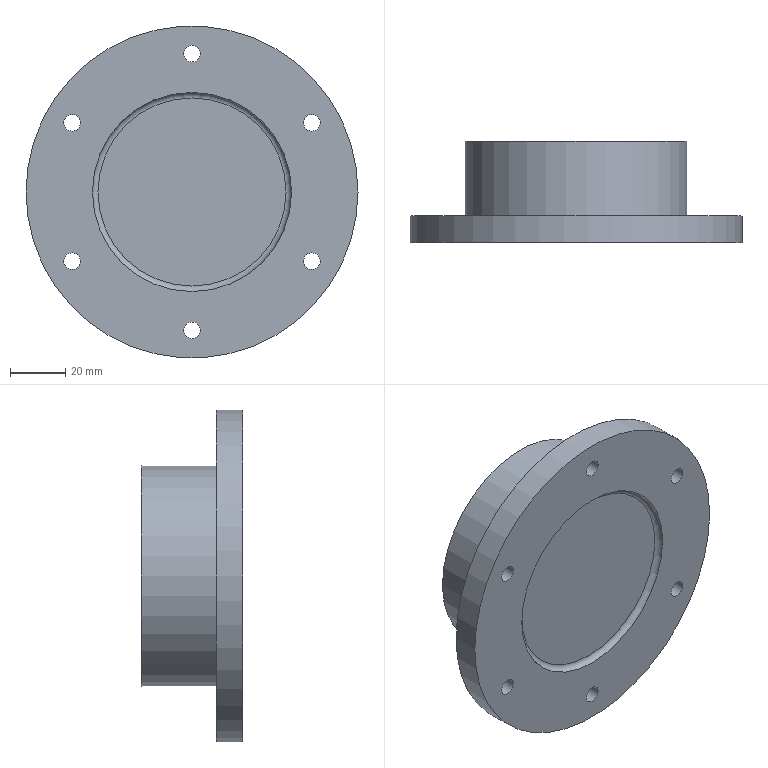Part | NX | features DATUM_CSYS 9, HOLE PACKAGE 9, SIMPLE HOLE 9, SKETCH 8, EXTRACT_DATUM_AXIS 6, EXTRACT_FACE 6, Instance Feature 5, BLEND 2, EXTRUDE 2, DELETE FACE 1, Pattern Feature 1 | 1 solid | 16 faces | box 120 x 36.6 x 120 mm | volume 144277 mm3 | cylinder 9 | plane 5 | torus 2 | commonest cylinder face diameters 6 x6 72 x1 80 x1 120 x1
STEP:
#1=CARTESIAN_POINT('',(60.,0.,0.));
#2=VERTEX_POINT('',#1);
#3=CARTESIAN_POINT('',(0.,0.,0.));
#4=DIRECTION('',(0.,-1.,0.));
#5=DIRECTION('',(1.,0.,0.));
#6=AXIS2_PLACEMENT_3D('',#3,#4,#5);
#7=CIRCLE('',#6,60.);
#8=EDGE_CURVE('',#2,#2,#7,.T.);
#9=ORIENTED_EDGE('',*,*,#8,.T.);
#10=EDGE_LOOP('',(#9));
#11=FACE_BOUND('',#10,.T.);
#12=CARTESIAN_POINT('',(60.,-9.6,0.));
#13=VERTEX_POINT('',#12);
#14=CARTESIAN_POINT('',(0.,-9.6,0.));
#15=DIRECTION('',(0.,-1.,0.));
#16=DIRECTION('',(1.,0.,0.));
#17=AXIS2_PLACEMENT_3D('',#14,#15,#16);
#18=CIRCLE('',#17,60.);
#19=EDGE_CURVE('',#13,#13,#18,.T.);
#20=ORIENTED_EDGE('',*,*,#19,.F.);
#21=EDGE_LOOP('',(#20));
#22=FACE_BOUND('',#21,.T.);
#23=CARTESIAN_POINT('',(0.,0.,0.));
#24=DIRECTION('',(0.,-1.,0.));
#25=DIRECTION('',(0.,0.,-1.));
#26=AXIS2_PLACEMENT_3D('',#23,#24,#25);
#27=CYLINDRICAL_SURFACE('',#26,60.);
#28=ADVANCED_FACE('',(#11,#22),#27,.T.);
#29=CARTESIAN_POINT('',(-43.301,0.,22.));
#30=VERTEX_POINT('',#29);
#31=CARTESIAN_POINT('',(-43.301,0.,25.));
#32=DIRECTION('',(0.,-1.,0.));
#33=DIRECTION('',(0.,0.,-1.));
#34=AXIS2_PLACEMENT_3D('',#31,#32,#33);
#35=CIRCLE('',#34,3.);
#36=EDGE_CURVE('',#30,#30,#35,.T.);
#37=ORIENTED_EDGE('',*,*,#36,.T.);
#38=EDGE_LOOP('',(#37));
#39=FACE_BOUND('',#38,.T.);
#40=CARTESIAN_POINT('',(-43.301,0.,-28.));
#41=VERTEX_POINT('',#40);
#42=CARTESIAN_POINT('',(-43.301,0.,-25.));
#43=DIRECTION('',(0.,-1.,0.));
#44=DIRECTION('',(0.,0.,-1.));
#45=AXIS2_PLACEMENT_3D('',#42,#43,#44);
#46=CIRCLE('',#45,3.);
#47=EDGE_CURVE('',#41,#41,#46,.T.);
#48=ORIENTED_EDGE('',*,*,#47,.T.);
#49=EDGE_LOOP('',(#48));
#50=FACE_BOUND('',#49,.T.);
#51=CARTESIAN_POINT('',(0.,0.,-53.));
#52=VERTEX_POINT('',#51);
#53=CARTESIAN_POINT('',(0.,0.,-50.));
#54=DIRECTION('',(0.,-1.,0.));
#55=DIRECTION('',(0.,0.,-1.));
#56=AXIS2_PLACEMENT_3D('',#53,#54,#55);
#57=CIRCLE('',#56,3.);
#58=EDGE_CURVE('',#52,#52,#57,.T.);
#59=ORIENTED_EDGE('',*,*,#58,.T.);
#60=EDGE_LOOP('',(#59));
#61=FACE_BOUND('',#60,.T.);
#62=CARTESIAN_POINT('',(43.301,0.,-28.));
#63=VERTEX_POINT('',#62);
#64=CARTESIAN_POINT('',(43.301,0.,-25.));
#65=DIRECTION('',(0.,-1.,0.));
#66=DIRECTION('',(0.,0.,-1.));
#67=AXIS2_PLACEMENT_3D('',#64,#65,#66);
#68=CIRCLE('',#67,3.);
#69=EDGE_CURVE('',#63,#63,#68,.T.);
#70=ORIENTED_EDGE('',*,*,#69,.T.);
#71=EDGE_LOOP('',(#70));
#72=FACE_BOUND('',#71,.T.);
#73=CARTESIAN_POINT('',(43.301,0.,22.));
#74=VERTEX_POINT('',#73);
#75=CARTESIAN_POINT('',(43.301,0.,25.));
#76=DIRECTION('',(0.,-1.,0.));
#77=DIRECTION('',(0.,0.,-1.));
#78=AXIS2_PLACEMENT_3D('',#75,#76,#77);
#79=CIRCLE('',#78,3.);
#80=EDGE_CURVE('',#74,#74,#79,.T.);
#81=ORIENTED_EDGE('',*,*,#80,.T.);
#82=EDGE_LOOP('',(#81));
#83=FACE_BOUND('',#82,.T.);
#84=CARTESIAN_POINT('',(0.,0.,47.));
#85=VERTEX_POINT('',#84);
#86=CARTESIAN_POINT('',(0.,0.,50.));
#87=DIRECTION('',(0.,-1.,0.));
#88=DIRECTION('',(0.,0.,-1.));
#89=AXIS2_PLACEMENT_3D('',#86,#87,#88);
#90=CIRCLE('',#89,3.);
#91=EDGE_CURVE('',#85,#85,#90,.T.);
#92=ORIENTED_EDGE('',*,*,#91,.T.);
#93=EDGE_LOOP('',(#92));
#94=FACE_BOUND('',#93,.T.);
#95=CARTESIAN_POINT('',(40.,0.,0.));
#96=VERTEX_POINT('',#95);
#97=CARTESIAN_POINT('',(0.,0.,0.));
#98=DIRECTION('',(0.,1.,0.));
#99=DIRECTION('',(1.,0.,0.));
#100=AXIS2_PLACEMENT_3D('',#97,#98,#99);
#101=CIRCLE('',#100,40.);
#102=EDGE_CURVE('',#96,#96,#101,.T.);
#103=ORIENTED_EDGE('',*,*,#102,.F.);
#104=EDGE_LOOP('',(#103));
#105=FACE_BOUND('',#104,.T.);
#106=ORIENTED_EDGE('',*,*,#8,.F.);
#107=EDGE_LOOP('',(#106));
#108=FACE_BOUND('',#107,.T.);
#109=CARTESIAN_POINT('',(0.,0.,0.));
#110=DIRECTION('',(0.,-1.,0.));
#111=DIRECTION('',(0.,0.,-1.));
#112=AXIS2_PLACEMENT_3D('',#109,#110,#111);
#113=PLANE('',#112);
#114=ADVANCED_FACE('',(#39,#50,#61,#72,#83,#94,#105,#108),#113,.F.);
#115=CARTESIAN_POINT('',(-43.301,-9.6,28.));
#116=VERTEX_POINT('',#115);
#117=CARTESIAN_POINT('',(-43.301,-9.6,25.));
#118=DIRECTION('',(0.,1.,0.));
#119=DIRECTION('',(0.,0.,1.));
#120=AXIS2_PLACEMENT_3D('',#117,#118,#119);
#121=CIRCLE('',#120,3.);
#122=EDGE_CURVE('',#116,#116,#121,.T.);
#123=ORIENTED_EDGE('',*,*,#122,.T.);
#124=EDGE_LOOP('',(#123));
#125=FACE_BOUND('',#124,.T.);
#126=CARTESIAN_POINT('',(-43.301,-9.6,-22.));
#127=VERTEX_POINT('',#126);
#128=CARTESIAN_POINT('',(-43.301,-9.6,-25.));
#129=DIRECTION('',(0.,1.,0.));
#130=DIRECTION('',(0.,0.,1.));
#131=AXIS2_PLACEMENT_3D('',#128,#129,#130);
#132=CIRCLE('',#131,3.);
#133=EDGE_CURVE('',#127,#127,#132,.T.);
#134=ORIENTED_EDGE('',*,*,#133,.T.);
#135=EDGE_LOOP('',(#134));
#136=FACE_BOUND('',#135,.T.);
#137=CARTESIAN_POINT('',(0.,-9.6,-47.));
#138=VERTEX_POINT('',#137);
#139=CARTESIAN_POINT('',(0.,-9.6,-50.));
#140=DIRECTION('',(0.,1.,0.));
#141=DIRECTION('',(0.,0.,1.));
#142=AXIS2_PLACEMENT_3D('',#139,#140,#141);
#143=CIRCLE('',#142,3.);
#144=EDGE_CURVE('',#138,#138,#143,.T.);
#145=ORIENTED_EDGE('',*,*,#144,.T.);
#146=EDGE_LOOP('',(#145));
#147=FACE_BOUND('',#146,.T.);
#148=CARTESIAN_POINT('',(43.301,-9.6,-22.));
#149=VERTEX_POINT('',#148);
#150=CARTESIAN_POINT('',(43.301,-9.6,-25.));
#151=DIRECTION('',(0.,1.,0.));
#152=DIRECTION('',(0.,0.,1.));
#153=AXIS2_PLACEMENT_3D('',#150,#151,#152);
#154=CIRCLE('',#153,3.);
#155=EDGE_CURVE('',#149,#149,#154,.T.);
#156=ORIENTED_EDGE('',*,*,#155,.T.);
#157=EDGE_LOOP('',(#156));
#158=FACE_BOUND('',#157,.T.);
#159=CARTESIAN_POINT('',(43.301,-9.6,28.));
#160=VERTEX_POINT('',#159);
#161=CARTESIAN_POINT('',(43.301,-9.6,25.));
#162=DIRECTION('',(0.,1.,0.));
#163=DIRECTION('',(0.,0.,1.));
#164=AXIS2_PLACEMENT_3D('',#161,#162,#163);
#165=CIRCLE('',#164,3.);
#166=EDGE_CURVE('',#160,#160,#165,.T.);
#167=ORIENTED_EDGE('',*,*,#166,.T.);
#168=EDGE_LOOP('',(#167));
#169=FACE_BOUND('',#168,.T.);
#170=CARTESIAN_POINT('',(0.,-9.6,53.));
#171=VERTEX_POINT('',#170);
#172=CARTESIAN_POINT('',(0.,-9.6,50.));
#173=DIRECTION('',(0.,1.,0.));
#174=DIRECTION('',(0.,0.,1.));
#175=AXIS2_PLACEMENT_3D('',#172,#173,#174);
#176=CIRCLE('',#175,3.);
#177=EDGE_CURVE('',#171,#171,#176,.T.);
#178=ORIENTED_EDGE('',*,*,#177,.T.);
#179=EDGE_LOOP('',(#178));
#180=FACE_BOUND('',#179,.T.);
#181=CARTESIAN_POINT('',(0.,-9.6,36.));
#182=VERTEX_POINT('',#181);
#183=CARTESIAN_POINT('',(0.,-9.6,0.));
#184=DIRECTION('',(0.,1.,0.));
#185=DIRECTION('',(0.,0.,1.));
#186=AXIS2_PLACEMENT_3D('',#183,#184,#185);
#187=CIRCLE('',#186,36.);
#188=EDGE_CURVE('',#182,#182,#187,.T.);
#189=ORIENTED_EDGE('',*,*,#188,.T.);
#190=EDGE_LOOP('',(#189));
#191=FACE_BOUND('',#190,.T.);
#192=ORIENTED_EDGE('',*,*,#19,.T.);
#193=EDGE_LOOP('',(#192));
#194=FACE_BOUND('',#193,.T.);
#195=CARTESIAN_POINT('',(0.,-9.6,0.));
#196=DIRECTION('',(0.,-1.,0.));
#197=DIRECTION('',(0.,0.,-1.));
#198=AXIS2_PLACEMENT_3D('',#195,#196,#197);
#199=PLANE('',#198);
#200=ADVANCED_FACE('',(#125,#136,#147,#158,#169,#180,#191,#194),#199,.T.);
#201=ORIENTED_EDGE('',*,*,#102,.T.);
#202=EDGE_LOOP('',(#201));
#203=FACE_BOUND('',#202,.T.);
#204=CARTESIAN_POINT('',(40.,27.,0.));
#205=VERTEX_POINT('',#204);
#206=CARTESIAN_POINT('',(0.,27.,0.));
#207=DIRECTION('',(0.,1.,0.));
#208=DIRECTION('',(1.,0.,0.));
#209=AXIS2_PLACEMENT_3D('',#206,#207,#208);
#210=CIRCLE('',#209,40.);
#211=EDGE_CURVE('',#205,#205,#210,.T.);
#212=ORIENTED_EDGE('',*,*,#211,.F.);
#213=EDGE_LOOP('',(#212));
#214=FACE_BOUND('',#213,.T.);
#215=CARTESIAN_POINT('',(0.,0.,0.));
#216=DIRECTION('',(0.,1.,0.));
#217=DIRECTION('',(0.,0.,1.));
#218=AXIS2_PLACEMENT_3D('',#215,#216,#217);
#219=CYLINDRICAL_SURFACE('',#218,40.);
#220=ADVANCED_FACE('',(#203,#214),#219,.T.);
#221=CARTESIAN_POINT('',(0.,27.,-36.));
#222=VERTEX_POINT('',#221);
#223=CARTESIAN_POINT('',(0.,27.,0.));
#224=DIRECTION('',(0.,-1.,0.));
#225=DIRECTION('',(0.,0.,-1.));
#226=AXIS2_PLACEMENT_3D('',#223,#224,#225);
#227=CIRCLE('',#226,36.);
#228=EDGE_CURVE('',#222,#222,#227,.T.);
#229=ORIENTED_EDGE('',*,*,#228,.T.);
#230=EDGE_LOOP('',(#229));
#231=FACE_BOUND('',#230,.T.);
#232=ORIENTED_EDGE('',*,*,#211,.T.);
#233=EDGE_LOOP('',(#232));
#234=FACE_BOUND('',#233,.T.);
#235=CARTESIAN_POINT('',(0.,27.,0.));
#236=DIRECTION('',(0.,1.,0.));
#237=DIRECTION('',(0.,0.,1.));
#238=AXIS2_PLACEMENT_3D('',#235,#236,#237);
#239=PLANE('',#238);
#240=ADVANCED_FACE('',(#231,#234),#239,.T.);
#241=CARTESIAN_POINT('',(0.,4.5,-31.));
#242=VERTEX_POINT('',#241);
#243=CARTESIAN_POINT('',(0.,4.5,0.));
#244=DIRECTION('',(0.,-1.,0.));
#245=DIRECTION('',(0.,0.,-1.));
#246=AXIS2_PLACEMENT_3D('',#243,#244,#245);
#247=CIRCLE('',#246,31.);
#248=EDGE_CURVE('',#242,#242,#247,.F.);
#249=ORIENTED_EDGE('',*,*,#248,.T.);
#250=EDGE_LOOP('',(#249));
#251=FACE_BOUND('',#250,.T.);
#252=CARTESIAN_POINT('',(0.,4.5,0.));
#253=DIRECTION('',(0.,-1.,0.));
#254=DIRECTION('',(0.,0.,-1.));
#255=AXIS2_PLACEMENT_3D('',#252,#253,#254);
#256=PLANE('',#255);
#257=ADVANCED_FACE('',(#251),#256,.F.);
#258=CARTESIAN_POINT('',(0.,9.5,-36.));
#259=VERTEX_POINT('',#258);
#260=CARTESIAN_POINT('',(0.,9.5,0.));
#261=DIRECTION('',(0.,-1.,0.));
#262=DIRECTION('',(0.,0.,-1.));
#263=AXIS2_PLACEMENT_3D('',#260,#261,#262);
#264=CIRCLE('',#263,36.);
#265=EDGE_CURVE('',#259,#259,#264,.T.);
#266=ORIENTED_EDGE('',*,*,#265,.T.);
#267=EDGE_LOOP('',(#266));
#268=FACE_BOUND('',#267,.T.);
#269=ORIENTED_EDGE('',*,*,#228,.F.);
#270=EDGE_LOOP('',(#269));
#271=FACE_BOUND('',#270,.T.);
#272=CARTESIAN_POINT('',(0.,27.,0.));
#273=DIRECTION('',(0.,-1.,0.));
#274=DIRECTION('',(0.,0.,-1.));
#275=AXIS2_PLACEMENT_3D('',#272,#273,#274);
#276=CYLINDRICAL_SURFACE('',#275,36.);
#277=ADVANCED_FACE('',(#268,#271),#276,.F.);
#278=CARTESIAN_POINT('',(0.,-7.6,34.));
#279=VERTEX_POINT('',#278);
#280=CARTESIAN_POINT('',(0.,-7.6,0.));
#281=DIRECTION('',(0.,1.,0.));
#282=DIRECTION('',(0.,0.,1.));
#283=AXIS2_PLACEMENT_3D('',#280,#281,#282);
#284=CIRCLE('',#283,34.);
#285=EDGE_CURVE('',#279,#279,#284,.F.);
#286=ORIENTED_EDGE('',*,*,#285,.T.);
#287=EDGE_LOOP('',(#286));
#288=FACE_BOUND('',#287,.T.);
#289=CARTESIAN_POINT('',(0.,-7.6,0.));
#290=DIRECTION('',(0.,1.,0.));
#291=DIRECTION('',(0.,0.,1.));
#292=AXIS2_PLACEMENT_3D('',#289,#290,#291);
#293=PLANE('',#292);
#294=ADVANCED_FACE('',(#288),#293,.F.);
#295=ORIENTED_EDGE('',*,*,#188,.F.);
#296=EDGE_LOOP('',(#295));
#297=FACE_BOUND('',#296,.T.);
#298=ORIENTED_EDGE('',*,*,#285,.F.);
#299=EDGE_LOOP('',(#298));
#300=FACE_BOUND('',#299,.T.);
#301=CARTESIAN_POINT('',(0.,-9.6,0.));
#302=DIRECTION('',(0.,1.,0.));
#303=DIRECTION('',(0.,0.,1.));
#304=AXIS2_PLACEMENT_3D('',#301,#302,#303);
#305=TOROIDAL_SURFACE('',#304,34.,2.);
#306=ADVANCED_FACE('',(#297,#300),#305,.F.);
#307=ORIENTED_EDGE('',*,*,#265,.F.);
#308=EDGE_LOOP('',(#307));
#309=FACE_BOUND('',#308,.T.);
#310=ORIENTED_EDGE('',*,*,#248,.F.);
#311=EDGE_LOOP('',(#310));
#312=FACE_BOUND('',#311,.T.);
#313=CARTESIAN_POINT('',(0.,9.5,0.));
#314=DIRECTION('',(0.,-1.,0.));
#315=DIRECTION('',(0.,0.,-1.));
#316=AXIS2_PLACEMENT_3D('',#313,#314,#315);
#317=TOROIDAL_SURFACE('',#316,31.,5.);
#318=ADVANCED_FACE('',(#309,#312),#317,.F.);
#319=ORIENTED_EDGE('',*,*,#177,.F.);
#320=EDGE_LOOP('',(#319));
#321=FACE_BOUND('',#320,.T.);
#322=ORIENTED_EDGE('',*,*,#91,.F.);
#323=EDGE_LOOP('',(#322));
#324=FACE_BOUND('',#323,.T.);
#325=CARTESIAN_POINT('',(0.,-9.6,50.));
#326=DIRECTION('',(0.,1.,0.));
#327=DIRECTION('',(0.,0.,1.));
#328=AXIS2_PLACEMENT_3D('',#325,#326,#327);
#329=CYLINDRICAL_SURFACE('',#328,3.);
#330=ADVANCED_FACE('',(#321,#324),#329,.F.);
#331=ORIENTED_EDGE('',*,*,#166,.F.);
#332=EDGE_LOOP('',(#331));
#333=FACE_BOUND('',#332,.T.);
#334=ORIENTED_EDGE('',*,*,#80,.F.);
#335=EDGE_LOOP('',(#334));
#336=FACE_BOUND('',#335,.T.);
#337=CARTESIAN_POINT('',(43.301,-9.6,25.));
#338=DIRECTION('',(0.,1.,0.));
#339=DIRECTION('',(0.,0.,1.));
#340=AXIS2_PLACEMENT_3D('',#337,#338,#339);
#341=CYLINDRICAL_SURFACE('',#340,3.);
#342=ADVANCED_FACE('',(#333,#336),#341,.F.);
#343=ORIENTED_EDGE('',*,*,#155,.F.);
#344=EDGE_LOOP('',(#343));
#345=FACE_BOUND('',#344,.T.);
#346=ORIENTED_EDGE('',*,*,#69,.F.);
#347=EDGE_LOOP('',(#346));
#348=FACE_BOUND('',#347,.T.);
#349=CARTESIAN_POINT('',(43.301,-9.6,-25.));
#350=DIRECTION('',(0.,1.,0.));
#351=DIRECTION('',(0.,0.,1.));
#352=AXIS2_PLACEMENT_3D('',#349,#350,#351);
#353=CYLINDRICAL_SURFACE('',#352,3.);
#354=ADVANCED_FACE('',(#345,#348),#353,.F.);
#355=ORIENTED_EDGE('',*,*,#144,.F.);
#356=EDGE_LOOP('',(#355));
#357=FACE_BOUND('',#356,.T.);
#358=ORIENTED_EDGE('',*,*,#58,.F.);
#359=EDGE_LOOP('',(#358));
#360=FACE_BOUND('',#359,.T.);
#361=CARTESIAN_POINT('',(0.,-9.6,-50.));
#362=DIRECTION('',(0.,1.,0.));
#363=DIRECTION('',(0.,0.,1.));
#364=AXIS2_PLACEMENT_3D('',#361,#362,#363);
#365=CYLINDRICAL_SURFACE('',#364,3.);
#366=ADVANCED_FACE('',(#357,#360),#365,.F.);
#367=ORIENTED_EDGE('',*,*,#133,.F.);
#368=EDGE_LOOP('',(#367));
#369=FACE_BOUND('',#368,.T.);
#370=ORIENTED_EDGE('',*,*,#47,.F.);
#371=EDGE_LOOP('',(#370));
#372=FACE_BOUND('',#371,.T.);
#373=CARTESIAN_POINT('',(-43.301,-9.6,-25.));
#374=DIRECTION('',(0.,1.,0.));
#375=DIRECTION('',(0.,0.,1.));
#376=AXIS2_PLACEMENT_3D('',#373,#374,#375);
#377=CYLINDRICAL_SURFACE('',#376,3.);
#378=ADVANCED_FACE('',(#369,#372),#377,.F.);
#379=ORIENTED_EDGE('',*,*,#122,.F.);
#380=EDGE_LOOP('',(#379));
#381=FACE_BOUND('',#380,.T.);
#382=ORIENTED_EDGE('',*,*,#36,.F.);
#383=EDGE_LOOP('',(#382));
#384=FACE_BOUND('',#383,.T.);
#385=CARTESIAN_POINT('',(-43.301,-9.6,25.));
#386=DIRECTION('',(0.,1.,0.));
#387=DIRECTION('',(0.,0.,1.));
#388=AXIS2_PLACEMENT_3D('',#385,#386,#387);
#389=CYLINDRICAL_SURFACE('',#388,3.);
#390=ADVANCED_FACE('',(#381,#384),#389,.F.);
#391=CLOSED_SHELL('',(#28,#114,#200,#220,#240,#257,#277,#294,#306,#318,#330,#342,#354,#366,#378,#390));
#392=MANIFOLD_SOLID_BREP('',#391);
#393=(LENGTH_UNIT()NAMED_UNIT(*)SI_UNIT(.MILLI.,.METRE.));
#394=UNCERTAINTY_MEASURE_WITH_UNIT(LENGTH_MEASURE(0.00001),#393,'','');
#395=(NAMED_UNIT(*)PLANE_ANGLE_UNIT()SI_UNIT($,.RADIAN.));
#396=(NAMED_UNIT(*)SI_UNIT($,.STERADIAN.)SOLID_ANGLE_UNIT());
#397=(GEOMETRIC_REPRESENTATION_CONTEXT(3)GLOBAL_UNCERTAINTY_ASSIGNED_CONTEXT((#394))GLOBAL_UNIT_ASSIGNED_CONTEXT((#393,#395,#396))REPRESENTATION_CONTEXT('',''));
#398=ADVANCED_BREP_SHAPE_REPRESENTATION('',(#392),#397);